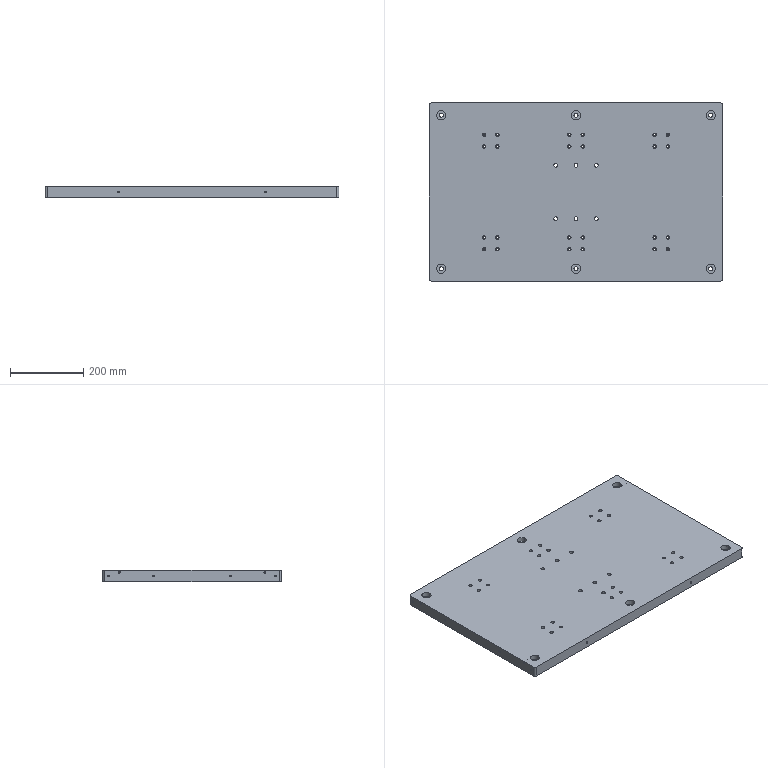NC program | Mastercam | posted with a generic post | part box 800 x 485 x 30 mm
Lines 5951 to 7047 of 7047:
N9930 T9 M6
N9940 G0 G90 G17 G54 X-367.93 Y210. A0. S6500 M3
N9950 G43 H9 Z50. M8
N9960 Z1.
N9970 G1 Z0. F600.
N9980 X-368.93 F2000.
N9990 G3 X-369.93 Y209. I0. J-1.
N100 X-367. Y206.07 Z-.125 I2.93 J0.
N110 X-364.07 Y209. Z-.25 I0. J2.93
N120 X-367. Y211.93 Z-.375 I-2.93 J0.
N130 X-369.93 Y209. Z-.5 I0. J-2.93
N140 X-367. Y206.07 Z-.625 I2.93 J0.
N150 X-364.07 Y209. Z-.75 I0. J2.93
N160 X-367. Y211.93 Z-.875 I-2.93 J0.
N170 X-369.93 Y209. Z-1. I0. J-2.93
N180 X-367. Y206.07 Z-1.125 I2.93 J0.
N190 X-364.07 Y209. Z-1.25 I0. J2.93
N200 X-367. Y211.93 Z-1.375 I-2.93 J0.
N210 X-369.93 Y209. Z-1.5 I0. J-2.93
N220 X-367. Y206.07 Z-1.625 I2.93 J0.
N230 X-364.07 Y209. Z-1.75 I0. J2.93
N240 X-367. Y211.93 Z-1.875 I-2.93 J0.
N250 X-369.93 Y209. Z-2. I0. J-2.93
N260 X-367. Y206.07 Z-2.125 I2.93 J0.
N270 X-364.07 Y209. Z-2.25 I0. J2.93
N280 X-367. Y211.93 Z-2.375 I-2.93 J0.
N290 X-369.93 Y209. Z-2.5 I0. J-2.93
N300 X-367. Y206.07 Z-2.625 I2.93 J0.
N310 X-364.07 Y209. Z-2.75 I0. J2.93
N320 X-367. Y211.93 Z-2.875 I-2.93 J0.
N330 X-369.93 Y209. Z-3. I0. J-2.93
N340 X-367. Y206.07 Z-3.125 I2.93 J0.
N350 X-364.07 Y209. Z-3.25 I0. J2.93
N360 X-367. Y211.93 Z-3.375 I-2.93 J0.
N370 X-369.93 Y209. Z-3.5 I0. J-2.93
N380 X-367. Y206.07 Z-3.625 I2.93 J0.
N390 X-364.07 Y209. Z-3.75 I0. J2.93
N400 X-367. Y211.93 Z-3.875 I-2.93 J0.
N410 X-369.93 Y209. Z-4. I0. J-2.93
N420 X-367. Y206.07 Z-4.125 I2.93 J0.
N430 X-364.07 Y209. Z-4.25 I0. J2.93
N440 X-367. Y211.93 Z-4.375 I-2.93 J0.
N450 X-369.93 Y209. Z-4.5 I0. J-2.93
N460 X-367. Y206.07 Z-4.625 I2.93 J0.
N470 X-364.07 Y209. Z-4.75 I0. J2.93
N480 X-367. Y211.93 Z-4.875 I-2.93 J0.
N490 X-369.93 Y209. Z-5. I0. J-2.93
N500 X-367. Y206.07 Z-5.125 I2.93 J0.
N510 X-364.07 Y209. Z-5.25 I0. J2.93
N520 X-367. Y211.93 Z-5.375 I-2.93 J0.
N530 X-369.93 Y209. Z-5.5 I0. J-2.93
N540 X-367. Y206.07 Z-5.625 I2.93 J0.
N550 X-364.07 Y209. Z-5.75 I0. J2.93
N560 X-367. Y211.93 Z-5.875 I-2.93 J0.
N570 X-369.93 Y209. Z-6. I0. J-2.93
N580 X-367. Y206.07 Z-6.125 I2.93 J0.
N590 X-364.07 Y209. Z-6.25 I0. J2.93
N600 X-367. Y211.93 Z-6.375 I-2.93 J0.
N610 X-369.93 Y209. Z-6.5 I0. J-2.93
N620 X-367. Y206.07 Z-6.625 I2.93 J0.
N630 X-364.07 Y209. Z-6.75 I0. J2.93
N640 X-367. Y211.93 Z-6.875 I-2.93 J0.
N650 X-369.93 Y209. Z-7. I0. J-2.93
N660 X-367. Y206.07 Z-7.125 I2.93 J0.
N670 X-364.07 Y209. Z-7.25 I0. J2.93
N680 X-367. Y211.93 Z-7.375 I-2.93 J0.
N690 X-369.93 Y209. Z-7.5 I0. J-2.93
N700 X-367. Y206.07 Z-7.625 I2.93 J0.
N710 X-364.07 Y209. Z-7.75 I0. J2.93
N720 X-367. Y211.93 Z-7.875 I-2.93 J0.
N730 X-369.93 Y209. Z-8. I0. J-2.93
N740 X-367. Y206.07 Z-8.125 I2.93 J0.
N750 X-364.07 Y209. Z-8.25 I0. J2.93
N760 X-367. Y211.93 Z-8.375 I-2.93 J0.
N770 X-369.93 Y209. Z-8.5 I0. J-2.93
N780 X-367. Y206.07 Z-8.625 I2.93 J0.
N790 X-364.07 Y209. Z-8.75 I0. J2.93
N800 X-367. Y211.93 Z-8.875 I-2.93 J0.
N810 X-369.93 Y209. Z-9. I0. J-2.93
N820 X-367. Y206.07 Z-9.125 I2.93 J0.
N830 X-364.07 Y209. Z-9.25 I0. J2.93
N840 X-367. Y211.93 Z-9.375 I-2.93 J0.
N850 X-369.93 Y209. Z-9.5 I0. J-2.93
N860 X-367. Y206.07 Z-9.625 I2.93 J0.
N870 X-364.07 Y209. Z-9.75 I0. J2.93
N880 X-367. Y211.93 Z-9.875 I-2.93 J0.
N890 X-369.93 Y209. Z-10. I0. J-2.93
N900 X-367. Y206.07 Z-10.125 I2.93 J0.
N910 X-364.07 Y209. Z-10.25 I0. J2.93
N920 X-367. Y211.93 Z-10.375 I-2.93 J0.
N930 X-369.93 Y209. Z-10.5 I0. J-2.93
N940 X-367. Y206.07 Z-10.625 I2.93 J0.
N950 X-364.07 Y209. Z-10.75 I0. J2.93
N960 X-367. Y211.93 Z-10.875 I-2.93 J0.
N970 X-369.37 Y210.722 Z-10.95 I0. J-2.93
N980 X-369.93 Y209. I2.37 J-1.722
N990 X-367. Y206.07 I2.93 J0.
N1000 X-364.07 Y209. I0. J2.93
N1010 X-367. Y211.93 I-2.93 J0.
N1020 X-369.37 Y210.722 I0. J-2.93
N1030 X-369.561 Y210.134 I.809 J-.588
N1040 X-369.149 Y209.325 I1. J0.
N1050 G1 X-368.34 Y208.738
N1060 G0 Z50.
N1070 X-367.93 Y-208.
N1080 Z1.
N1090 G1 Z0. F600.
N1100 X-368.93 F2000.
N1110 G3 X-369.93 Y-209. I0. J-1.
N1120 X-367. Y-211.93 Z-.125 I2.93 J0.
N1130 X-364.07 Y-209. Z-.25 I0. J2.93
N1140 X-367. Y-206.07 Z-.375 I-2.93 J0.
N1150 X-369.93 Y-209. Z-.5 I0. J-2.93
N1160 X-367. Y-211.93 Z-.625 I2.93 J0.
N1170 X-364.07 Y-209. Z-.75 I0. J2.93
N1180 X-367. Y-206.07 Z-.875 I-2.93 J0.
N1190 X-369.93 Y-209. Z-1. I0. J-2.93
N1200 X-367. Y-211.93 Z-1.125 I2.93 J0.
N1210 X-364.07 Y-209. Z-1.25 I0. J2.93
N1220 X-367. Y-206.07 Z-1.375 I-2.93 J0.
N1230 X-369.93 Y-209. Z-1.5 I0. J-2.93
N1240 X-367. Y-211.93 Z-1.625 I2.93 J0.
N1250 X-364.07 Y-209. Z-1.75 I0. J2.93
N1260 X-367. Y-206.07 Z-1.875 I-2.93 J0.
N1270 X-369.93 Y-209. Z-2. I0. J-2.93
N1280 X-367. Y-211.93 Z-2.125 I2.93 J0.
N1290 X-364.07 Y-209. Z-2.25 I0. J2.93
N1300 X-367. Y-206.07 Z-2.375 I-2.93 J0.
N1310 X-369.93 Y-209. Z-2.5 I0. J-2.93
N1320 X-367. Y-211.93 Z-2.625 I2.93 J0.
N1330 X-364.07 Y-209. Z-2.75 I0. J2.93
N1340 X-367. Y-206.07 Z-2.875 I-2.93 J0.
N1350 X-369.93 Y-209. Z-3. I0. J-2.93
N1360 X-367. Y-211.93 Z-3.125 I2.93 J0.
N1370 X-364.07 Y-209. Z-3.25 I0. J2.93
N1380 X-367. Y-206.07 Z-3.375 I-2.93 J0.
N1390 X-369.93 Y-209. Z-3.5 I0. J-2.93
N1400 X-367. Y-211.93 Z-3.625 I2.93 J0.
N1410 X-364.07 Y-209. Z-3.75 I0. J2.93
N1420 X-367. Y-206.07 Z-3.875 I-2.93 J0.
N1430 X-369.93 Y-209. Z-4. I0. J-2.93
N1440 X-367. Y-211.93 Z-4.125 I2.93 J0.
N1450 X-364.07 Y-209. Z-4.25 I0. J2.93
N1460 X-367. Y-206.07 Z-4.375 I-2.93 J0.
N1470 X-369.93 Y-209. Z-4.5 I0. J-2.93
N1480 X-367. Y-211.93 Z-4.625 I2.93 J0.
N1490 X-364.07 Y-209. Z-4.75 I0. J2.93
N1500 X-367. Y-206.07 Z-4.875 I-2.93 J0.
N1510 X-369.93 Y-209. Z-5. I0. J-2.93
N1520 X-367. Y-211.93 Z-5.125 I2.93 J0.
N1530 X-364.07 Y-209. Z-5.25 I0. J2.93
N1540 X-367. Y-206.07 Z-5.375 I-2.93 J0.
N1550 X-369.93 Y-209. Z-5.5 I0. J-2.93
N1560 X-367. Y-211.93 Z-5.625 I2.93 J0.
N1570 X-364.07 Y-209. Z-5.75 I0. J2.93
N1580 X-367. Y-206.07 Z-5.875 I-2.93 J0.
N1590 X-369.93 Y-209. Z-6. I0. J-2.93
N1600 X-367. Y-211.93 Z-6.125 I2.93 J0.
N1610 X-364.07 Y-209. Z-6.25 I0. J2.93
N1620 X-367. Y-206.07 Z-6.375 I-2.93 J0.
N1630 X-369.93 Y-209. Z-6.5 I0. J-2.93
N1640 X-367. Y-211.93 Z-6.625 I2.93 J0.
N1650 X-364.07 Y-209. Z-6.75 I0. J2.93
N1660 X-367. Y-206.07 Z-6.875 I-2.93 J0.
N1670 X-369.93 Y-209. Z-7. I0. J-2.93
N1680 X-367. Y-211.93 Z-7.125 I2.93 J0.
N1690 X-364.07 Y-209. Z-7.25 I0. J2.93
N1700 X-367. Y-206.07 Z-7.375 I-2.93 J0.
N1710 X-369.93 Y-209. Z-7.5 I0. J-2.93
N1720 X-367. Y-211.93 Z-7.625 I2.93 J0.
N1730 X-364.07 Y-209. Z-7.75 I0. J2.93
N1740 X-367. Y-206.07 Z-7.875 I-2.93 J0.
N1750 X-369.93 Y-209. Z-8. I0. J-2.93
N1760 X-367. Y-211.93 Z-8.125 I2.93 J0.
N1770 X-364.07 Y-209. Z-8.25 I0. J2.93
N1780 X-367. Y-206.07 Z-8.375 I-2.93 J0.
N1790 X-369.93 Y-209. Z-8.5 I0. J-2.93
N1800 X-367. Y-211.93 Z-8.625 I2.93 J0.
N1810 X-364.07 Y-209. Z-8.75 I0. J2.93
N1820 X-367. Y-206.07 Z-8.875 I-2.93 J0.
N1830 X-369.93 Y-209. Z-9. I0. J-2.93
N1840 X-367. Y-211.93 Z-9.125 I2.93 J0.
N1850 X-364.07 Y-209. Z-9.25 I0. J2.93
N1860 X-367. Y-206.07 Z-9.375 I-2.93 J0.
N1870 X-369.93 Y-209. Z-9.5 I0. J-2.93
N1880 X-367. Y-211.93 Z-9.625 I2.93 J0.
N1890 X-364.07 Y-209. Z-9.75 I0. J2.93
N1900 X-367. Y-206.07 Z-9.875 I-2.93 J0.
N1910 X-369.93 Y-209. Z-10. I0. J-2.93
N1920 X-367. Y-211.93 Z-10.125 I2.93 J0.
N1930 X-364.07 Y-209. Z-10.25 I0. J2.93
N1940 X-367. Y-206.07 Z-10.375 I-2.93 J0.
N1950 X-369.93 Y-209. Z-10.5 I0. J-2.93
N1960 X-367. Y-211.93 Z-10.625 I2.93 J0.
N1970 X-364.07 Y-209. Z-10.75 I0. J2.93
N1980 X-367. Y-206.07 Z-10.875 I-2.93 J0.
N1990 X-369.37 Y-207.278 Z-10.95 I0. J-2.93
N2000 X-369.93 Y-209. I2.37 J-1.722
N2010 X-367. Y-211.93 I2.93 J0.
N2020 X-364.07 Y-209. I0. J2.93
N2030 X-367. Y-206.07 I-2.93 J0.
N2040 X-369.37 Y-207.278 I0. J-2.93
N2050 X-369.561 Y-207.866 I.809 J-.588
N2060 X-369.149 Y-208.675 I1. J0.
N2070 G1 X-368.34 Y-209.262
N2080 G0 Z50.
N2090 X-.93 Y-208.
N2100 Z1.
N2110 G1 Z0. F600.
N2120 X-1.93 F2000.
N2130 G3 X-2.93 Y-209. I0. J-1.
N2140 X0. Y-211.93 Z-.125 I2.93 J0.
N2150 X2.93 Y-209. Z-.25 I0. J2.93
N2160 X0. Y-206.07 Z-.375 I-2.93 J0.
N2170 X-2.93 Y-209. Z-.5 I0. J-2.93
N2180 X0. Y-211.93 Z-.625 I2.93 J0.
N2190 X2.93 Y-209. Z-.75 I0. J2.93
N2200 X0. Y-206.07 Z-.875 I-2.93 J0.
N2210 X-2.93 Y-209. Z-1. I0. J-2.93
N2220 X0. Y-211.93 Z-1.125 I2.93 J0.
N2230 X2.93 Y-209. Z-1.25 I0. J2.93
N2240 X0. Y-206.07 Z-1.375 I-2.93 J0.
N2250 X-2.93 Y-209. Z-1.5 I0. J-2.93
N2260 X0. Y-211.93 Z-1.625 I2.93 J0.
N2270 X2.93 Y-209. Z-1.75 I0. J2.93
N2280 X0. Y-206.07 Z-1.875 I-2.93 J0.
N2290 X-2.93 Y-209. Z-2. I0. J-2.93
N2300 X0. Y-211.93 Z-2.125 I2.93 J0.
N2310 X2.93 Y-209. Z-2.25 I0. J2.93
N2320 X0. Y-206.07 Z-2.375 I-2.93 J0.
N2330 X-2.93 Y-209. Z-2.5 I0. J-2.93
N2340 X0. Y-211.93 Z-2.625 I2.93 J0.
N2350 X2.93 Y-209. Z-2.75 I0. J2.93
N2360 X0. Y-206.07 Z-2.875 I-2.93 J0.
N2370 X-2.93 Y-209. Z-3. I0. J-2.93
N2380 X0. Y-211.93 Z-3.125 I2.93 J0.
N2390 X2.93 Y-209. Z-3.25 I0. J2.93
N2400 X0. Y-206.07 Z-3.375 I-2.93 J0.
N2410 X-2.93 Y-209. Z-3.5 I0. J-2.93
N2420 X0. Y-211.93 Z-3.625 I2.93 J0.
N2430 X2.93 Y-209. Z-3.75 I0. J2.93
N2440 X0. Y-206.07 Z-3.875 I-2.93 J0.
N2450 X-2.93 Y-209. Z-4. I0. J-2.93
N2460 X0. Y-211.93 Z-4.125 I2.93 J0.
N2470 X2.93 Y-209. Z-4.25 I0. J2.93
N2480 X0. Y-206.07 Z-4.375 I-2.93 J0.
N2490 X-2.93 Y-209. Z-4.5 I0. J-2.93
N2500 X0. Y-211.93 Z-4.625 I2.93 J0.
N2510 X2.93 Y-209. Z-4.75 I0. J2.93
N2520 X0. Y-206.07 Z-4.875 I-2.93 J0.
N2530 X-2.93 Y-209. Z-5. I0. J-2.93
N2540 X0. Y-211.93 Z-5.125 I2.93 J0.
N2550 X2.93 Y-209. Z-5.25 I0. J2.93
N2560 X0. Y-206.07 Z-5.375 I-2.93 J0.
N2570 X-2.93 Y-209. Z-5.5 I0. J-2.93
N2580 X0. Y-211.93 Z-5.625 I2.93 J0.
N2590 X2.93 Y-209. Z-5.75 I0. J2.93
N2600 X0. Y-206.07 Z-5.875 I-2.93 J0.
N2610 X-2.93 Y-209. Z-6. I0. J-2.93
N2620 X0. Y-211.93 Z-6.125 I2.93 J0.
N2630 X2.93 Y-209. Z-6.25 I0. J2.93
N2640 X0. Y-206.07 Z-6.375 I-2.93 J0.
N2650 X-2.93 Y-209. Z-6.5 I0. J-2.93
N2660 X0. Y-211.93 Z-6.625 I2.93 J0.
N2670 X2.93 Y-209. Z-6.75 I0. J2.93
N2680 X0. Y-206.07 Z-6.875 I-2.93 J0.
N2690 X-2.93 Y-209. Z-7. I0. J-2.93
N2700 X0. Y-211.93 Z-7.125 I2.93 J0.
N2710 X2.93 Y-209. Z-7.25 I0. J2.93
N2720 X0. Y-206.07 Z-7.375 I-2.93 J0.
N2730 X-2.93 Y-209. Z-7.5 I0. J-2.93
N2740 X0. Y-211.93 Z-7.625 I2.93 J0.
N2750 X2.93 Y-209. Z-7.75 I0. J2.93
N2760 X0. Y-206.07 Z-7.875 I-2.93 J0.
N2770 X-2.93 Y-209. Z-8. I0. J-2.93
N2780 X0. Y-211.93 Z-8.125 I2.93 J0.
N2790 X2.93 Y-209. Z-8.25 I0. J2.93
N2800 X0. Y-206.07 Z-8.375 I-2.93 J0.
N2810 X-2.93 Y-209. Z-8.5 I0. J-2.93
N2820 X0. Y-211.93 Z-8.625 I2.93 J0.
N2830 X2.93 Y-209. Z-8.75 I0. J2.93
N2840 X0. Y-206.07 Z-8.875 I-2.93 J0.
N2850 X-2.93 Y-209. Z-9. I0. J-2.93
N2860 X0. Y-211.93 Z-9.125 I2.93 J0.
N2870 X2.93 Y-209. Z-9.25 I0. J2.93
N2880 X0. Y-206.07 Z-9.375 I-2.93 J0.
N2890 X-2.93 Y-209. Z-9.5 I0. J-2.93
N2900 X0. Y-211.93 Z-9.625 I2.93 J0.
N2910 X2.93 Y-209. Z-9.75 I0. J2.93
N2920 X0. Y-206.07 Z-9.875 I-2.93 J0.
N2930 X-2.93 Y-209. Z-10. I0. J-2.93
N2940 X0. Y-211.93 Z-10.125 I2.93 J0.
N2950 X2.93 Y-209. Z-10.25 I0. J2.93
N2960 X0. Y-206.07 Z-10.375 I-2.93 J0.
N2970 X-2.93 Y-209. Z-10.5 I0. J-2.93
N2980 X0. Y-211.93 Z-10.625 I2.93 J0.
N2990 X2.93 Y-209. Z-10.75 I0. J2.93
N3000 X0. Y-206.07 Z-10.875 I-2.93 J0.
N3010 X-2.37 Y-207.278 Z-10.95 I0. J-2.93
N3020 X-2.93 Y-209. I2.37 J-1.722
N3030 X0. Y-211.93 I2.93 J0.
N3040 X2.93 Y-209. I0. J2.93
N3050 X0. Y-206.07 I-2.93 J0.
N3060 X-2.37 Y-207.278 I0. J-2.93
N3070 X-2.561 Y-207.866 I.809 J-.588
N3080 X-2.149 Y-208.675 I1. J0.
N3090 G1 X-1.34 Y-209.262
N3100 G0 Z50.
N3110 X366.07 Y-208.
N3120 Z1.
N3130 G1 Z0. F600.
N3140 X365.07 F2000.
N3150 G3 X364.07 Y-209. I0. J-1.
N3160 X367. Y-211.93 Z-.125 I2.93 J0.
N3170 X369.93 Y-209. Z-.25 I0. J2.93
N3180 X367. Y-206.07 Z-.375 I-2.93 J0.
N3190 X364.07 Y-209. Z-.5 I0. J-2.93
N3200 X367. Y-211.93 Z-.625 I2.93 J0.
N3210 X369.93 Y-209. Z-.75 I0. J2.93
N3220 X367. Y-206.07 Z-.875 I-2.93 J0.
N3230 X364.07 Y-209. Z-1. I0. J-2.93
N3240 X367. Y-211.93 Z-1.125 I2.93 J0.
N3250 X369.93 Y-209. Z-1.25 I0. J2.93
N3260 X367. Y-206.07 Z-1.375 I-2.93 J0.
N3270 X364.07 Y-209. Z-1.5 I0. J-2.93
N3280 X367. Y-211.93 Z-1.625 I2.93 J0.
N3290 X369.93 Y-209. Z-1.75 I0. J2.93
N3300 X367. Y-206.07 Z-1.875 I-2.93 J0.
N3310 X364.07 Y-209. Z-2. I0. J-2.93
N3320 X367. Y-211.93 Z-2.125 I2.93 J0.
N3330 X369.93 Y-209. Z-2.25 I0. J2.93
N3340 X367. Y-206.07 Z-2.375 I-2.93 J0.
N3350 X364.07 Y-209. Z-2.5 I0. J-2.93
N3360 X367. Y-211.93 Z-2.625 I2.93 J0.
N3370 X369.93 Y-209. Z-2.75 I0. J2.93
N3380 X367. Y-206.07 Z-2.875 I-2.93 J0.
N3390 X364.07 Y-209. Z-3. I0. J-2.93
N3400 X367. Y-211.93 Z-3.125 I2.93 J0.
N3410 X369.93 Y-209. Z-3.25 I0. J2.93
N3420 X367. Y-206.07 Z-3.375 I-2.93 J0.
N3430 X364.07 Y-209. Z-3.5 I0. J-2.93
N3440 X367. Y-211.93 Z-3.625 I2.93 J0.
N3450 X369.93 Y-209. Z-3.75 I0. J2.93
N3460 X367. Y-206.07 Z-3.875 I-2.93 J0.
N3470 X364.07 Y-209. Z-4. I0. J-2.93
N3480 X367. Y-211.93 Z-4.125 I2.93 J0.
N3490 X369.93 Y-209. Z-4.25 I0. J2.93
N3500 X367. Y-206.07 Z-4.375 I-2.93 J0.
N3510 X364.07 Y-209. Z-4.5 I0. J-2.93
N3520 X367. Y-211.93 Z-4.625 I2.93 J0.
N3530 X369.93 Y-209. Z-4.75 I0. J2.93
N3540 X367. Y-206.07 Z-4.875 I-2.93 J0.
N3550 X364.07 Y-209. Z-5. I0. J-2.93
N3560 X367. Y-211.93 Z-5.125 I2.93 J0.
N3570 X369.93 Y-209. Z-5.25 I0. J2.93
N3580 X367. Y-206.07 Z-5.375 I-2.93 J0.
N3590 X364.07 Y-209. Z-5.5 I0. J-2.93
N3600 X367. Y-211.93 Z-5.625 I2.93 J0.
N3610 X369.93 Y-209. Z-5.75 I0. J2.93
N3620 X367. Y-206.07 Z-5.875 I-2.93 J0.
N3630 X364.07 Y-209. Z-6. I0. J-2.93
N3640 X367. Y-211.93 Z-6.125 I2.93 J0.
N3650 X369.93 Y-209. Z-6.25 I0. J2.93
N3660 X367. Y-206.07 Z-6.375 I-2.93 J0.
N3670 X364.07 Y-209. Z-6.5 I0. J-2.93
N3680 X367. Y-211.93 Z-6.625 I2.93 J0.
N3690 X369.93 Y-209. Z-6.75 I0. J2.93
N3700 X367. Y-206.07 Z-6.875 I-2.93 J0.
N3710 X364.07 Y-209. Z-7. I0. J-2.93
N3720 X367. Y-211.93 Z-7.125 I2.93 J0.
N3730 X369.93 Y-209. Z-7.25 I0. J2.93
N3740 X367. Y-206.07 Z-7.375 I-2.93 J0.
N3750 X364.07 Y-209. Z-7.5 I0. J-2.93
N3760 X367. Y-211.93 Z-7.625 I2.93 J0.
N3770 X369.93 Y-209. Z-7.75 I0. J2.93
N3780 X367. Y-206.07 Z-7.875 I-2.93 J0.
N3790 X364.07 Y-209. Z-8. I0. J-2.93
N3800 X367. Y-211.93 Z-8.125 I2.93 J0.
N3810 X369.93 Y-209. Z-8.25 I0. J2.93
N3820 X367. Y-206.07 Z-8.375 I-2.93 J0.
N3830 X364.07 Y-209. Z-8.5 I0. J-2.93
N3840 X367. Y-211.93 Z-8.625 I2.93 J0.
N3850 X369.93 Y-209. Z-8.75 I0. J2.93
N3860 X367. Y-206.07 Z-8.875 I-2.93 J0.
N3870 X364.07 Y-209. Z-9. I0. J-2.93
N3880 X367. Y-211.93 Z-9.125 I2.93 J0.
N3890 X369.93 Y-209. Z-9.25 I0. J2.93
N3900 X367. Y-206.07 Z-9.375 I-2.93 J0.
N3910 X364.07 Y-209. Z-9.5 I0. J-2.93
N3920 X367. Y-211.93 Z-9.625 I2.93 J0.
N3930 X369.93 Y-209. Z-9.75 I0. J2.93
N3940 X367. Y-206.07 Z-9.875 I-2.93 J0.
N3950 X364.07 Y-209. Z-10. I0. J-2.93
N3960 X367. Y-211.93 Z-10.125 I2.93 J0.
N3970 X369.93 Y-209. Z-10.25 I0. J2.93
N3980 X367. Y-206.07 Z-10.375 I-2.93 J0.
N3990 X364.07 Y-209. Z-10.5 I0. J-2.93
N4000 X367. Y-211.93 Z-10.625 I2.93 J0.
N4010 X369.93 Y-209. Z-10.75 I0. J2.93
N4020 X367. Y-206.07 Z-10.875 I-2.93 J0.
N4030 X364.63 Y-207.278 Z-10.95 I0. J-2.93
N4040 X364.07 Y-209. I2.37 J-1.722
N4050 X367. Y-211.93 I2.93 J0.
N4060 X369.93 Y-209. I0. J2.93
N4070 X367. Y-206.07 I-2.93 J0.
N4080 X364.63 Y-207.278 I0. J-2.93
N4090 X364.439 Y-207.866 I.809 J-.588
N4100 X364.851 Y-208.675 I1. J0.
N4110 G1 X365.66 Y-209.262
N4120 G0 Z50.
N4130 X366.07 Y210.
N4140 Z1.
N4150 G1 Z0. F600.
N4160 X365.07 F2000.
N4170 G3 X364.07 Y209. I0. J-1.
N4180 X367. Y206.07 Z-.125 I2.93 J0.
N4190 X369.93 Y209. Z-.25 I0. J2.93
N4200 X367. Y211.93 Z-.375 I-2.93 J0.
N4210 X364.07 Y209. Z-.5 I0. J-2.93
N4220 X367. Y206.07 Z-.625 I2.93 J0.
N4230 X369.93 Y209. Z-.75 I0. J2.93
N4240 X367. Y211.93 Z-.875 I-2.93 J0.
N4250 X364.07 Y209. Z-1. I0. J-2.93
N4260 X367. Y206.07 Z-1.125 I2.93 J0.
N4270 X369.93 Y209. Z-1.25 I0. J2.93
N4280 X367. Y211.93 Z-1.375 I-2.93 J0.
N4290 X364.07 Y209. Z-1.5 I0. J-2.93
N4300 X367. Y206.07 Z-1.625 I2.93 J0.
N4310 X369.93 Y209. Z-1.75 I0. J2.93
N4320 X367. Y211.93 Z-1.875 I-2.93 J0.
N4330 X364.07 Y209. Z-2. I0. J-2.93
N4340 X367. Y206.07 Z-2.125 I2.93 J0.
N4350 X369.93 Y209. Z-2.25 I0. J2.93
N4360 X367. Y211.93 Z-2.375 I-2.93 J0.
N4370 X364.07 Y209. Z-2.5 I0. J-2.93
N4380 X367. Y206.07 Z-2.625 I2.93 J0.
N4390 X369.93 Y209. Z-2.75 I0. J2.93
N4400 X367. Y211.93 Z-2.875 I-2.93 J0.
N4410 X364.07 Y209. Z-3. I0. J-2.93
N4420 X367. Y206.07 Z-3.125 I2.93 J0.
N4430 X369.93 Y209. Z-3.25 I0. J2.93
N4440 X367. Y211.93 Z-3.375 I-2.93 J0.
N4450 X364.07 Y209. Z-3.5 I0. J-2.93
N4460 X367. Y206.07 Z-3.625 I2.93 J0.
N4470 X369.93 Y209. Z-3.75 I0. J2.93
N4480 X367. Y211.93 Z-3.875 I-2.93 J0.
N4490 X364.07 Y209. Z-4. I0. J-2.93
N4500 X367. Y206.07 Z-4.125 I2.93 J0.
N4510 X369.93 Y209. Z-4.25 I0. J2.93
N4520 X367. Y211.93 Z-4.375 I-2.93 J0.
N4530 X364.07 Y209. Z-4.5 I0. J-2.93
N4540 X367. Y206.07 Z-4.625 I2.93 J0.
N4550 X369.93 Y209. Z-4.75 I0. J2.93
N4560 X367. Y211.93 Z-4.875 I-2.93 J0.
N4570 X364.07 Y209. Z-5. I0. J-2.93
N4580 X367. Y206.07 Z-5.125 I2.93 J0.
N4590 X369.93 Y209. Z-5.25 I0. J2.93
N4600 X367. Y211.93 Z-5.375 I-2.93 J0.
N4610 X364.07 Y209. Z-5.5 I0. J-2.93
N4620 X367. Y206.07 Z-5.625 I2.93 J0.
N4630 X369.93 Y209. Z-5.75 I0. J2.93
N4640 X367. Y211.93 Z-5.875 I-2.93 J0.
N4650 X364.07 Y209. Z-6. I0. J-2.93
N4660 X367. Y206.07 Z-6.125 I2.93 J0.
N4670 X369.93 Y209. Z-6.25 I0. J2.93
N4680 X367. Y211.93 Z-6.375 I-2.93 J0.
N4690 X364.07 Y209. Z-6.5 I0. J-2.93
N4700 X367. Y206.07 Z-6.625 I2.93 J0.
N4710 X369.93 Y209. Z-6.75 I0. J2.93
N4720 X367. Y211.93 Z-6.875 I-2.93 J0.
N4730 X364.07 Y209. Z-7. I0. J-2.93
N4740 X367. Y206.07 Z-7.125 I2.93 J0.
N4750 X369.93 Y209. Z-7.25 I0. J2.93
N4760 X367. Y211.93 Z-7.375 I-2.93 J0.
N4770 X364.07 Y209. Z-7.5 I0. J-2.93
N4780 X367. Y206.07 Z-7.625 I2.93 J0.
N4790 X369.93 Y209. Z-7.75 I0. J2.93
N4800 X367. Y211.93 Z-7.875 I-2.93 J0.
N4810 X364.07 Y209. Z-8. I0. J-2.93
N4820 X367. Y206.07 Z-8.125 I2.93 J0.
N4830 X369.93 Y209. Z-8.25 I0. J2.93
N4840 X367. Y211.93 Z-8.375 I-2.93 J0.
N4850 X364.07 Y209. Z-8.5 I0. J-2.93
N4860 X367. Y206.07 Z-8.625 I2.93 J0.
N4870 X369.93 Y209. Z-8.75 I0. J2.93
N4880 X367. Y211.93 Z-8.875 I-2.93 J0.
N4890 X364.07 Y209. Z-9. I0. J-2.93
N4900 X367. Y206.07 Z-9.125 I2.93 J0.
N4910 X369.93 Y209. Z-9.25 I0. J2.93
N4920 X367. Y211.93 Z-9.375 I-2.93 J0.
N4930 X364.07 Y209. Z-9.5 I0. J-2.93
N4940 X367. Y206.07 Z-9.625 I2.93 J0.
N4950 X369.93 Y209. Z-9.75 I0. J2.93
N4960 X367. Y211.93 Z-9.875 I-2.93 J0.
N4970 X364.07 Y209. Z-10. I0. J-2.93
N4980 X367. Y206.07 Z-10.125 I2.93 J0.
N4990 X369.93 Y209. Z-10.25 I0. J2.93
N5000 X367. Y211.93 Z-10.375 I-2.93 J0.
N5010 X364.07 Y209. Z-10.5 I0. J-2.93
N5020 X367. Y206.07 Z-10.625 I2.93 J0.
N5030 X369.93 Y209. Z-10.75 I0. J2.93
N5040 X367. Y211.93 Z-10.875 I-2.93 J0.
N5050 X364.63 Y210.722 Z-10.95 I0. J-2.93
N5060 X364.07 Y209. I2.37 J-1.722
N5070 X367. Y206.07 I2.93 J0.
N5080 X369.93 Y209. I0. J2.93
N5090 X367. Y211.93 I-2.93 J0.
N5100 X364.63 Y210.722 I0. J-2.93
N5110 X364.439 Y210.134 I.809 J-.588
N5120 X364.851 Y209.325 I1. J0.
N5130 G1 X365.66 Y208.738
N5140 G0 Z50.
N5150 X-.93 Y210.
N5160 Z1.
N5170 G1 Z0. F600.
N5180 X-1.93 F2000.
N5190 G3 X-2.93 Y209. I0. J-1.
N5200 X0. Y206.07 Z-.125 I2.93 J0.
N5210 X2.93 Y209. Z-.25 I0. J2.93
N5220 X0. Y211.93 Z-.375 I-2.93 J0.
N5230 X-2.93 Y209. Z-.5 I0. J-2.93
N5240 X0. Y206.07 Z-.625 I2.93 J0.
N5250 X2.93 Y209. Z-.75 I0. J2.93
N5260 X0. Y211.93 Z-.875 I-2.93 J0.
N5270 X-2.93 Y209. Z-1. I0. J-2.93
N5280 X0. Y206.07 Z-1.125 I2.93 J0.
N5290 X2.93 Y209. Z-1.25 I0. J2.93
N5300 X0. Y211.93 Z-1.375 I-2.93 J0.
N5310 X-2.93 Y209. Z-1.5 I0. J-2.93
N5320 X0. Y206.07 Z-1.625 I2.93 J0.
N5330 X2.93 Y209. Z-1.75 I0. J2.93
N5340 X0. Y211.93 Z-1.875 I-2.93 J0.
N5350 X-2.93 Y209. Z-2. I0. J-2.93
N5360 X0. Y206.07 Z-2.125 I2.93 J0.
N5370 X2.93 Y209. Z-2.25 I0. J2.93
N5380 X0. Y211.93 Z-2.375 I-2.93 J0.
N5390 X-2.93 Y209. Z-2.5 I0. J-2.93
N5400 X0. Y206.07 Z-2.625 I2.93 J0.
N5410 X2.93 Y209. Z-2.75 I0. J2.93
N5420 X0. Y211.93 Z-2.875 I-2.93 J0.
N5430 X-2.93 Y209. Z-3. I0. J-2.93
N5440 X0. Y206.07 Z-3.125 I2.93 J0.
N5450 X2.93 Y209. Z-3.25 I0. J2.93
N5460 X0. Y211.93 Z-3.375 I-2.93 J0.
N5470 X-2.93 Y209. Z-3.5 I0. J-2.93
N5480 X0. Y206.07 Z-3.625 I2.93 J0.
N5490 X2.93 Y209. Z-3.75 I0. J2.93
N5500 X0. Y211.93 Z-3.875 I-2.93 J0.
N5510 X-2.93 Y209. Z-4. I0. J-2.93
N5520 X0. Y206.07 Z-4.125 I2.93 J0.
N5530 X2.93 Y209. Z-4.25 I0. J2.93
N5540 X0. Y211.93 Z-4.375 I-2.93 J0.
N5550 X-2.93 Y209. Z-4.5 I0. J-2.93
N5560 X0. Y206.07 Z-4.625 I2.93 J0.
N5570 X2.93 Y209. Z-4.75 I0. J2.93
N5580 X0. Y211.93 Z-4.875 I-2.93 J0.
N5590 X-2.93 Y209. Z-5. I0. J-2.93
N5600 X0. Y206.07 Z-5.125 I2.93 J0.
N5610 X2.93 Y209. Z-5.25 I0. J2.93
N5620 X0. Y211.93 Z-5.375 I-2.93 J0.
N5630 X-2.93 Y209. Z-5.5 I0. J-2.93
N5640 X0. Y206.07 Z-5.625 I2.93 J0.
N5650 X2.93 Y209. Z-5.75 I0. J2.93
N5660 X0. Y211.93 Z-5.875 I-2.93 J0.
N5670 X-2.93 Y209. Z-6. I0. J-2.93
N5680 X0. Y206.07 Z-6.125 I2.93 J0.
N5690 X2.93 Y209. Z-6.25 I0. J2.93
N5700 X0. Y211.93 Z-6.375 I-2.93 J0.
N5710 X-2.93 Y209. Z-6.5 I0. J-2.93
N5720 X0. Y206.07 Z-6.625 I2.93 J0.
N5730 X2.93 Y209. Z-6.75 I0. J2.93
N5740 X0. Y211.93 Z-6.875 I-2.93 J0.
N5750 X-2.93 Y209. Z-7. I0. J-2.93
N5760 X0. Y206.07 Z-7.125 I2.93 J0.
N5770 X2.93 Y209. Z-7.25 I0. J2.93
N5780 X0. Y211.93 Z-7.375 I-2.93 J0.
N5790 X-2.93 Y209. Z-7.5 I0. J-2.93
N5800 X0. Y206.07 Z-7.625 I2.93 J0.
N5810 X2.93 Y209. Z-7.75 I0. J2.93
N5820 X0. Y211.93 Z-7.875 I-2.93 J0.
N5830 X-2.93 Y209. Z-8. I0. J-2.93
N5840 X0. Y206.07 Z-8.125 I2.93 J0.
N5850 X2.93 Y209. Z-8.25 I0. J2.93
N5860 X0. Y211.93 Z-8.375 I-2.93 J0.
N5870 X-2.93 Y209. Z-8.5 I0. J-2.93
N5880 X0. Y206.07 Z-8.625 I2.93 J0.
N5890 X2.93 Y209. Z-8.75 I0. J2.93
N5900 X0. Y211.93 Z-8.875 I-2.93 J0.
N5910 X-2.93 Y209. Z-9. I0. J-2.93
N5920 X0. Y206.07 Z-9.125 I2.93 J0.
N5930 X2.93 Y209. Z-9.25 I0. J2.93
N5940 X0. Y211.93 Z-9.375 I-2.93 J0.
N5950 X-2.93 Y209. Z-9.5 I0. J-2.93
N5960 X0. Y206.07 Z-9.625 I2.93 J0.
N5970 X2.93 Y209. Z-9.75 I0. J2.93
N5980 X0. Y211.93 Z-9.875 I-2.93 J0.
N5990 X-2.93 Y209. Z-10. I0. J-2.93
N6000 X0. Y206.07 Z-10.125 I2.93 J0.
N6010 X2.93 Y209. Z-10.25 I0. J2.93
N6020 X0. Y211.93 Z-10.375 I-2.93 J0.
N6030 X-2.93 Y209. Z-10.5 I0. J-2.93
N6040 X0. Y206.07 Z-10.625 I2.93 J0.
N6050 X2.93 Y209. Z-10.75 I0. J2.93
N6060 X0. Y211.93 Z-10.875 I-2.93 J0.
N6070 X-2.37 Y210.722 Z-10.95 I0. J-2.93
N6080 X-2.93 Y209. I2.37 J-1.722
N6090 X0. Y206.07 I2.93 J0.
N6100 X2.93 Y209. I0. J2.93
N6110 X0. Y211.93 I-2.93 J0.
N6120 X-2.37 Y210.722 I0. J-2.93
N6130 X-2.561 Y210.134 I.809 J-.588
N6140 X-2.149 Y209.325 I1. J0.
N6150 G1 X-1.34 Y208.738
N6160 G0 Z50.
N6170 M5
N6180 G91 G28 Z0. M9
N6190 A0.
N6200 M01
N6210 T10 M6
N6220 G0 G90 G17 G54 X-368. Y210. A0. S6500 M3
N6230 G43 H10 Z50. M8
N6240 Z1.
N6250 G1 Z-11. F600.
N6260 X-369. F1000.
N6270 G3 X-370. Y209. I0. J-1.
N6280 X-367. Y206. I3. J0.
N6290 X-364. Y209. I0. J3.
N6300 X-367. Y212. I-3. J0.
N6310 X-370. Y209. I0. J-3.
N6320 X-369. Y208. I1. J0.
N6330 G1 X-368.
N6340 G0 Z50.
N6350 Y-208.
N6360 Z1.
N6370 G1 Z-11. F600.
N6380 X-369. F1000.
N6390 G3 X-370. Y-209. I0. J-1.
N6400 X-367. Y-212. I3. J0.
N6410 X-364. Y-209. I0. J3.
N6420 X-367. Y-206. I-3. J0.
N6430 X-370. Y-209. I0. J-3.
N6440 X-369. Y-210. I1. J0.
N6450 G1 X-368.
N6460 G0 Z50.
N6470 X-1. Y-208.
N6480 Z1.
N6490 G1 Z-11. F600.
N6500 X-2. F1000.
N6510 G3 X-3. Y-209. I0. J-1.
N6520 X0. Y-212. I3. J0.
N6530 X3. Y-209. I0. J3.
N6540 X0. Y-206. I-3. J0.
N6550 X-3. Y-209. I0. J-3.
N6560 X-2. Y-210. I1. J0.
N6570 G1 X-1.
N6580 G0 Z50.
N6590 X366. Y-208.
N6600 Z1.
N6610 G1 Z-11. F600.
N6620 X365. F1000.
N6630 G3 X364. Y-209. I0. J-1.
N6640 X367. Y-212. I3. J0.
N6650 X370. Y-209. I0. J3.
N6660 X367. Y-206. I-3. J0.
N6670 X364. Y-209. I0. J-3.
N6680 X365. Y-210. I1. J0.
N6690 G1 X366.
N6700 G0 Z50.
N6710 Y210.
N6720 Z1.
N6730 G1 Z-11. F600.
N6740 X365. F1000.
N6750 G3 X364. Y209. I0. J-1.
N6760 X367. Y206. I3. J0.
N6770 X370. Y209. I0. J3.
N6780 X367. Y212. I-3. J0.
N6790 X364. Y209. I0. J-3.
N6800 X365. Y208. I1. J0.
N6810 G1 X366.
N6820 G0 Z50.
N6830 X-1. Y210.
N6840 Z1.
N6850 G1 Z-11. F600.
N6860 X-2. F1000.
N6870 G3 X-3. Y209. I0. J-1.
N6880 X0. Y206. I3. J0.
N6890 X3. Y209. I0. J3.
N6900 X0. Y212. I-3. J0.
N6910 X-3. Y209. I0. J-3.
N6920 X-2. Y208. I1. J0.
N6930 G1 X-1.
N6940 G0 Z50.
N6950 M5
N6960 G91 G28 Z0. M9
N6970 A0.
N6980 M01
N6990 T7 M6
N7000 G0 G90 G17 G54 X-373.55 Y209.4 A0. S6000 M3
N7010 G43 H7 Z50. M8
N7020 Z1.
N7030 G1 Z-.75 F600.
N7040 X-373.95 F1000.
N7050 G3 X-374.35 Y209. I0. J-.4
N7060 X-367. Y201.65 I7.35 J0.
N7070 X-359.65 Y209. I0. J7.35
N7080 X-367. Y216.35 I-7.35 J0.
N7090 X-374.35 Y209. I0. J-7.35
N7100 X-373.95 Y208.6 I.4 J0.
N7110 G1 X-373.55
N7120 G0 Z50.
N7130 Y-208.6
N7140 Z1.
N7150 G1 Z-.75 F600.
N7160 X-373.95 F1000.
N7170 G3 X-374.35 Y-209. I0. J-.4
N7180 X-367. Y-216.35 I7.35 J0.
N7190 X-359.65 Y-209. I0. J7.35
N7200 X-367. Y-201.65 I-7.35 J0.
N7210 X-374.35 Y-209. I0. J-7.35
N7220 X-373.95 Y-209.4 I.4 J0.
N7230 G1 X-373.55
N7240 G0 Z50.
N7250 X-6.55 Y-208.6
N7260 Z1.
N7270 G1 Z-.75 F600.
N7280 X-6.95 F1000.
N7290 G3 X-7.35 Y-209. I0. J-.4
N7300 X0. Y-216.35 I7.35 J0.
N7310 X7.35 Y-209. I0. J7.35
N7320 X0. Y-201.65 I-7.35 J0.
N7330 X-7.35 Y-209. I0. J-7.35
N7340 X-6.95 Y-209.4 I.4 J0.
N7350 G1 X-6.55
N7360 G0 Z50.
N7370 X360.45 Y-208.6
N7380 Z1.
N7390 G1 Z-.75 F600.
N7400 X360.05 F1000.
N7410 G3 X359.65 Y-209. I0. J-.4
N7420 X367. Y-216.35 I7.35 J0.
N7430 X374.35 Y-209. I0. J7.35
N7440 X367. Y-201.65 I-7.35 J0.
N7450 X359.65 Y-209. I0. J-7.35
N7460 X360.05 Y-209.4 I.4 J0.
N7470 G1 X360.45
N7480 G0 Z50.
N7490 Y209.4
N7500 Z1.
N7510 G1 Z-.75 F600.
N7520 X360.05 F1000.
N7530 G3 X359.65 Y209. I0. J-.4
N7540 X367. Y201.65 I7.35 J0.
N7550 X374.35 Y209. I0. J7.35
N7560 X367. Y216.35 I-7.35 J0.
N7570 X359.65 Y209. I0. J-7.35
N7580 X360.05 Y208.6 I.4 J0.
N7590 G1 X360.45
N7600 G0 Z50.
N7610 X-6.55 Y209.4
N7620 Z1.
N7630 G1 Z-.75 F600.
N7640 X-6.95 F1000.
N7650 G3 X-7.35 Y209. I0. J-.4
N7660 X0. Y201.65 I7.35 J0.
N7670 X7.35 Y209. I0. J7.35
N7680 X0. Y216.35 I-7.35 J0.
N7690 X-7.35 Y209. I0. J-7.35
N7700 X-6.95 Y208.6 I.4 J0.
N7710 G1 X-6.55
N7720 G0 Z50.
N7730 X-371.05 Y209.4
N7740 Z-10.
N7750 G1 Z-11.75 F600.
N7760 X-371.45 F1000.
N7770 G3 X-371.85 Y209. I0. J-.4
N7780 X-367. Y204.15 I4.85 J0.
N7790 X-362.15 Y209. I0. J4.85
N7800 X-367. Y213.85 I-4.85 J0.
N7810 X-371.85 Y209. I0. J-4.85
N7820 X-371.45 Y208.6 I.4 J0.
N7830 G1 X-371.05
N7840 G0 Z50.
N7850 X-4.05 Y209.4
N7860 Z-10.
N7870 G1 Z-11.75 F600.
N7880 X-4.45 F1000.
N7890 G3 X-4.85 Y209. I0. J-.4
N7900 X0. Y204.15 I4.85 J0.
N7910 X4.85 Y209. I0. J4.85
N7920 X0. Y213.85 I-4.85 J0.
N7930 X-4.85 Y209. I0. J-4.85
N7940 X-4.45 Y208.6 I.4 J0.
N7950 G1 X-4.05
N7960 G0 Z50.
N7970 X362.95 Y209.4
N7980 Z-10.
N7990 G1 Z-11.75 F600.
N8000 X362.55 F1000.
N8010 G3 X362.15 Y209. I0. J-.4
N8020 X367. Y204.15 I4.85 J0.
N8030 X371.85 Y209. I0. J4.85
N8040 X367. Y213.85 I-4.85 J0.
N8050 X362.15 Y209. I0. J-4.85
N8060 X362.55 Y208.6 I.4 J0.
N8070 G1 X362.95
N8080 G0 Z50.
N8090 Y-208.6
N8100 Z-10.
N8110 G1 Z-11.75 F600.
N8120 X362.55 F1000.
N8130 G3 X362.15 Y-209. I0. J-.4
N8140 X367. Y-213.85 I4.85 J0.
N8150 X371.85 Y-209. I0. J4.85
N8160 X367. Y-204.15 I-4.85 J0.
N8170 X362.15 Y-209. I0. J-4.85
N8180 X362.55 Y-209.4 I.4 J0.
N8190 G1 X362.95
N8200 G0 Z50.
N8210 X-4.05 Y-208.6
N8220 Z-10.
N8230 G1 Z-11.75 F600.
N8240 X-4.45 F1000.
N8250 G3 X-4.85 Y-209. I0. J-.4
N8260 X0. Y-213.85 I4.85 J0.
N8270 X4.85 Y-209. I0. J4.85
N8280 X0. Y-204.15 I-4.85 J0.
N8290 X-4.85 Y-209. I0. J-4.85
N8300 X-4.45 Y-209.4 I.4 J0.
N8310 G1 X-4.05
N8320 G0 Z50.
N8330 X-371.05 Y-208.6
N8340 Z-10.
N8350 G1 Z-11.75 F600.
N8360 X-371.45 F1000.
N8370 G3 X-371.85 Y-209. I0. J-.4
N8380 X-367. Y-213.85 I4.85 J0.
N8390 X-362.15 Y-209. I0. J4.85
N8400 X-367. Y-204.15 I-4.85 J0.
N8410 X-371.85 Y-209. I0. J-4.85
N8420 X-371.45 Y-209.4 I.4 J0.
N8430 G1 X-371.05
N8440 G0 Z50.
N8450 X-200. Y0.
N8460 G98 G81 Z-.7 R1. F200.
N8470 X200.
N8480 G80
N8490 M5
N8500 G91 G0 G28 Z0. M9
N8510 A0.
N8520 M01
N8530 T18 M6
N8540 G0 G90 G17 G54 X-200. Y0. A0. S1200 M3
N8550 G43 H18 Z50. M8
N8560 G98 G83 Z-22. R1. Q2. F100.
N8570 X200.
N8580 G80
N8590 M5
N8600 G91 G0 G28 Z0. M9
N8610 A0.
N8620 M01
N8630 T7 M6
N8640 G0 G90 G17 G54 X-201.05 Y.4 A0. S6000 M3
N8650 G43 H7 Z50. M8
N8660 Z1.
N8670 G1 Z-1. F600.
N8680 X-201.45 F1000.
N8690 G3 X-201.85 Y0. I0. J-.4
N8700 X-200. Y-1.85 I1.85 J0.
N8710 X-198.15 Y0. I0. J1.85
N8720 X-200. Y1.85 I-1.85 J0.
N8730 X-201.85 Y0. I0. J-1.85
N8740 X-201.45 Y-.4 I.4 J0.
N8750 G1 X-201.05
N8760 G0 Z50.
N8770 X198.95 Y.4
N8780 Z1.
N8790 G1 Z-1. F600.
N8800 X198.55 F1000.
N8810 G3 X198.15 Y0. I0. J-.4
N8820 X200. Y-1.85 I1.85 J0.
N8830 X201.85 Y0. I0. J1.85
N8840 X200. Y1.85 I-1.85 J0.
N8850 X198.15 Y0. I0. J-1.85
N8860 X198.55 Y-.4 I.4 J0.
N8870 G1 X198.95
N8880 G0 Z50.
N8890 X227.5 Y0.
N8900 G98 G81 Z-.7 R1. F200.
N8910 X198.5 Y-10.
N8920 X105. Y0.
N8930 X-105.
N8940 X-198.5 Y-10.
N8950 X-227.5 Y0.
N8960 G80
N8970 M5
N8980 G91 G0 G28 Z0. M9
N8990 A0.
N9000 M01
N9010 T15 M6
N9020 G0 G90 G17 G54 X227.5 Y0. A0. S1200 M3
N9030 G43 H15 Z50. M8
N9040 G98 G83 Z-20. R1. Q2. F100.
N9050 X198.5 Y-10.
N9060 X105. Y0.
N9070 X-105.
N9080 X-198.5 Y-10.
N9090 X-227.5 Y0.
N9100 G80
N9110 M5
N9120 G91 G0 G28 Z0. M9
N9130 A0.
N9140 M01
N9150 T7 M6
N9160 G0 G90 G17 G54 X-228.65 Y.4 A0. S6000 M3
N9170 G43 H7 Z50. M8
N9180 Z1.
N9190 G1 Z-1. F600.
N9200 X-229.05 F1000.
N9210 G3 X-229.45 Y0. I0. J-.4
N9220 X-227.5 Y-1.95 I1.95 J0.
N9230 X-225.55 Y0. I0. J1.95
N9240 X-227.5 Y1.95 I-1.95 J0.
N9250 X-229.45 Y0. I0. J-1.95
N9260 X-229.05 Y-.4 I.4 J0.
N9270 G1 X-228.65
N9280 G0 Z50.
N9290 X197.35 Y-9.6
N9300 Z1.
N9310 G1 Z-1. F600.
N9320 X196.95 F1000.
N9330 G3 X196.55 Y-10. I0. J-.4
N9340 X198.5 Y-11.95 I1.95 J0.
N9350 X200.45 Y-10. I0. J1.95
N9360 X198.5 Y-8.05 I-1.95 J0.
N9370 X196.55 Y-10. I0. J-1.95
N9380 X196.95 Y-10.4 I.4 J0.
N9390 G1 X197.35
N9400 G0 Z50.
N9410 X226.35 Y.4
N9420 Z1.
N9430 G1 Z-1. F600.
N9440 X225.95 F1000.
N9450 G3 X225.55 Y0. I0. J-.4
N9460 X227.5 Y-1.95 I1.95 J0.
N9470 X229.45 Y0. I0. J1.95
N9480 X227.5 Y1.95 I-1.95 J0.
N9490 X225.55 Y0. I0. J-1.95
N9500 X225.95 Y-.4 I.4 J0.
N9510 G1 X226.35
N9520 G0 Z50.
N9530 X103.85 Y.4
N9540 Z1.
N9550 G1 Z-1. F600.
N9560 X103.45 F1000.
N9570 G3 X103.05 Y0. I0. J-.4
N9580 X105. Y-1.95 I1.95 J0.
N9590 X106.95 Y0. I0. J1.95
N9600 X105. Y1.95 I-1.95 J0.
N9610 X103.05 Y0. I0. J-1.95
N9620 X103.45 Y-.4 I.4 J0.
N9630 G1 X103.85
N9640 G0 Z50.
N9650 X-106.15 Y.4
N9660 Z1.
N9670 G1 Z-1. F600.
N9680 X-106.55 F1000.
N9690 G3 X-106.95 Y0. I0. J-.4
N9700 X-105. Y-1.95 I1.95 J0.
N9710 X-103.05 Y0. I0. J1.95
N9720 X-105. Y1.95 I-1.95 J0.
N9730 X-106.95 Y0. I0. J-1.95
N9740 X-106.55 Y-.4 I.4 J0.
N9750 G1 X-106.15
N9760 G0 Z50.
N9770 X-199.65 Y-9.6
N9780 Z1.
N9790 G1 Z-1. F600.
N9800 X-200.05 F1000.
N9810 G3 X-200.45 Y-10. I0. J-.4
N9820 X-198.5 Y-11.95 I1.95 J0.
N9830 X-196.55 Y-10. I0. J1.95
N9840 X-198.5 Y-8.05 I-1.95 J0.
N9850 X-200.45 Y-10. I0. J-1.95
N9860 X-200.05 Y-10.4 I.4 J0.
N9870 G1 X-199.65
N9880 G0 Z50.
N9890 M5
N9900 G91 G28 Z0. M9
N9910 A0.
N9920 M01
N9930 T10 M6
N9940 G0 G90 G17 G54 X3. Y208. A0. S6500 M3
N9950 G43 H10 Z50. M8
N9960 Z1.
N9970 G1 Z0. F600.
N9980 X4. F1500.
N9990 G3 X5. Y209. I0. J1.
N100 X0. Y214. Z-.125 I-5. J0.
N110 X-5. Y209. Z-.25 I0. J-5.
N120 X0. Y204. Z-.375 I5. J0.
N130 X5. Y209. Z-.5 I0. J5.
N140 X0. Y214. Z-.625 I-5. J0.
N150 X-5. Y209. Z-.75 I0. J-5.
N160 X0. Y204. Z-.875 I5. J0.
N170 X5. Y209. Z-1. I0. J5.
N180 X0. Y214. Z-1.125 I-5. J0.
N190 X-5. Y209. Z-1.25 I0. J-5.
N200 X0. Y204. Z-1.375 I5. J0.
N210 X5. Y209. Z-1.5 I0. J5.
N220 X0. Y214. Z-1.625 I-5. J0.
N230 X-5. Y209. Z-1.75 I0. J-5.
N240 X0. Y204. Z-1.875 I5. J0.
N250 X5. Y209. Z-2. I0. J5.
N260 X0. Y214. Z-2.125 I-5. J0.
N270 X-5. Y209. Z-2.25 I0. J-5.
N280 X0. Y204. Z-2.375 I5. J0.
N290 X5. Y209. Z-2.5 I0. J5.
N300 X0. Y214. Z-2.625 I-5. J0.
N310 X-5. Y209. Z-2.75 I0. J-5.
N320 X0. Y204. Z-2.875 I5. J0.
N330 X5. Y209. Z-3. I0. J5.
N340 X0. Y214. Z-3.125 I-5. J0.
N350 X-5. Y209. Z-3.25 I0. J-5.
N360 X0. Y204. Z-3.375 I5. J0.
N370 X5. Y209. Z-3.5 I0. J5.
N380 X0. Y214. Z-3.625 I-5. J0.
N390 X-5. Y209. Z-3.75 I0. J-5.
N400 X0. Y204. Z-3.875 I5. J0.
N410 X5. Y209. Z-4. I0. J5.
N420 X0. Y214. Z-4.125 I-5. J0.
N430 X-5. Y209. Z-4.25 I0. J-5.
N440 X0. Y204. Z-4.375 I5. J0.
N450 X5. Y209. Z-4.5 I0. J5.
N460 X0. Y214. Z-4.625 I-5. J0.
N470 X-5. Y209. Z-4.75 I0. J-5.
N480 X0. Y204. Z-4.875 I5. J0.
N490 X5. Y209. Z-5. I0. J5.
N500 X0. Y214. Z-5.125 I-5. J0.
N510 X-5. Y209. Z-5.25 I0. J-5.
N520 X0. Y204. Z-5.375 I5. J0.
N530 X5. Y209. Z-5.5 I0. J5.
N540 X0. Y214. Z-5.625 I-5. J0.
N550 X-5. Y209. Z-5.75 I0. J-5.
N560 X0. Y204. Z-5.875 I5. J0.
N570 X5. Y209. Z-6. I0. J5.
N580 X0. Y214. Z-6.125 I-5. J0.
N590 X-5. Y209. Z-6.25 I0. J-5.
N600 X0. Y204. Z-6.375 I5. J0.
N610 X5. Y209. Z-6.5 I0. J5.
N620 X0. Y214. Z-6.625 I-5. J0.
N630 X-5. Y209. Z-6.75 I0. J-5.
N640 X0. Y204. Z-6.875 I5. J0.
N650 X5. Y209. Z-7. I0. J5.
N660 X0. Y214. Z-7.125 I-5. J0.
N670 X-5. Y209. Z-7.25 I0. J-5.
N680 X0. Y204. Z-7.375 I5. J0.
N690 X5. Y209. Z-7.5 I0. J5.
N700 X0. Y214. Z-7.625 I-5. J0.
N710 X-5. Y209. Z-7.75 I0. J-5.
N720 X0. Y204. Z-7.875 I5. J0.
N730 X5. Y209. Z-8. I0. J5.
N740 X0. Y214. Z-8.125 I-5. J0.
N750 X-5. Y209. Z-8.25 I0. J-5.
N760 X0. Y204. Z-8.375 I5. J0.
N770 X5. Y209. Z-8.5 I0. J5.
N780 X0. Y214. Z-8.625 I-5. J0.
N790 X-5. Y209. Z-8.75 I0. J-5.
N800 X0. Y204. Z-8.875 I5. J0.
N810 X5. Y209. Z-9. I0. J5.
N820 X0. Y214. Z-9.125 I-5. J0.
N830 X-5. Y209. Z-9.25 I0. J-5.
N840 X0. Y204. Z-9.375 I5. J0.
N850 X5. Y209. Z-9.5 I0. J5.
N860 X0. Y214. Z-9.625 I-5. J0.
N870 X-5. Y209. Z-9.75 I0. J-5.
N880 X0. Y204. Z-9.875 I5. J0.
N890 X5. Y209. Z-10. I0. J5.
N900 X0. Y214. Z-10.125 I-5. J0.
N910 X-5. Y209. Z-10.25 I0. J-5.
N920 X0. Y204. Z-10.375 I5. J0.
N930 X5. Y209. Z-10.5 I0. J5.
N940 X0. Y214. Z-10.625 I-5. J0.
N950 X-5. Y209. Z-10.75 I0. J-5.
N960 X0. Y204. Z-10.875 I5. J0.
N970 X5. Y209. Z-11. I0. J5.
N980 X0. Y214. I-5. J0.
N990 X-5. Y209. I0. J-5.
N1000 X0. Y204. I5. J0.
N1010 X5. Y209. I0. J5.
N1020 X4. Y210. I-1. J0.
N1030 G1 X3.
N1040 G0 Z50.
N1050 M5
N1060 G91 G28 Z0. M9
N1070 G28 X0. Y0. A0.
N1080 M30
%